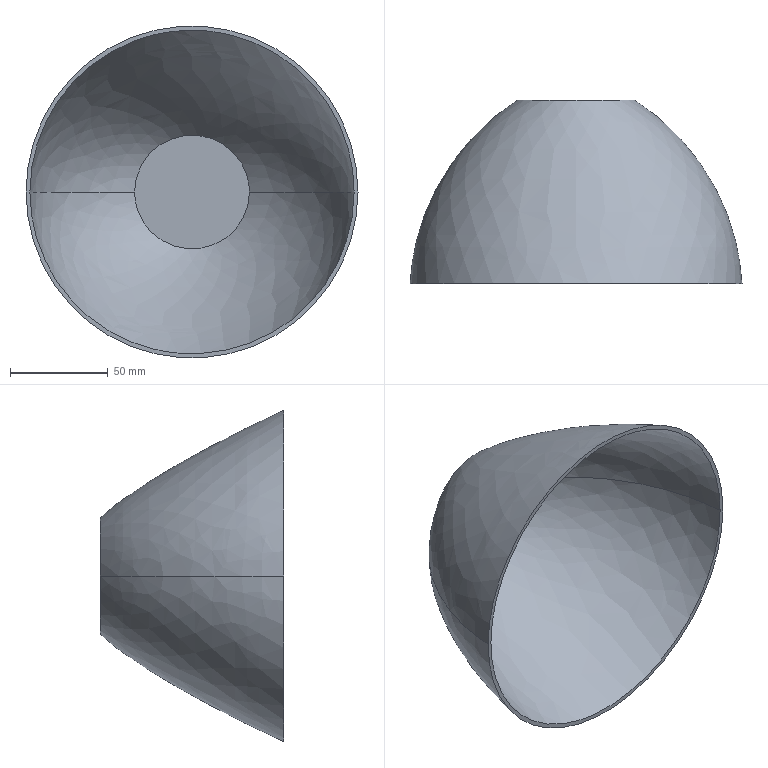Part | SolidWorks | features Blend 1, Shell 1 | 1 solid | 7 faces | box 170 x 94.745 x 170 mm | volume 90040 mm3 | spline 4 | plane 3